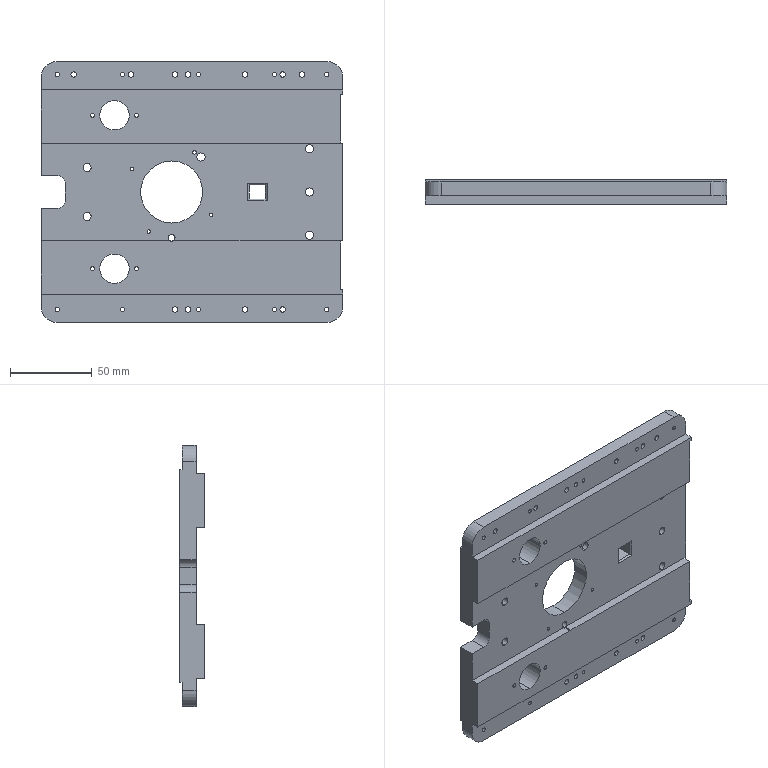Part | STEP file | PN_0007 Default | 1 solid | 139 faces | box 185 x 15 x 160 mm | volume 319731 mm3 | cylinder 92 | plane 39 | cone 8 | commonest cylinder face diameters 2.5 x36 3.3 x22 5 x12 2.05 x8 18 x4 20 x4